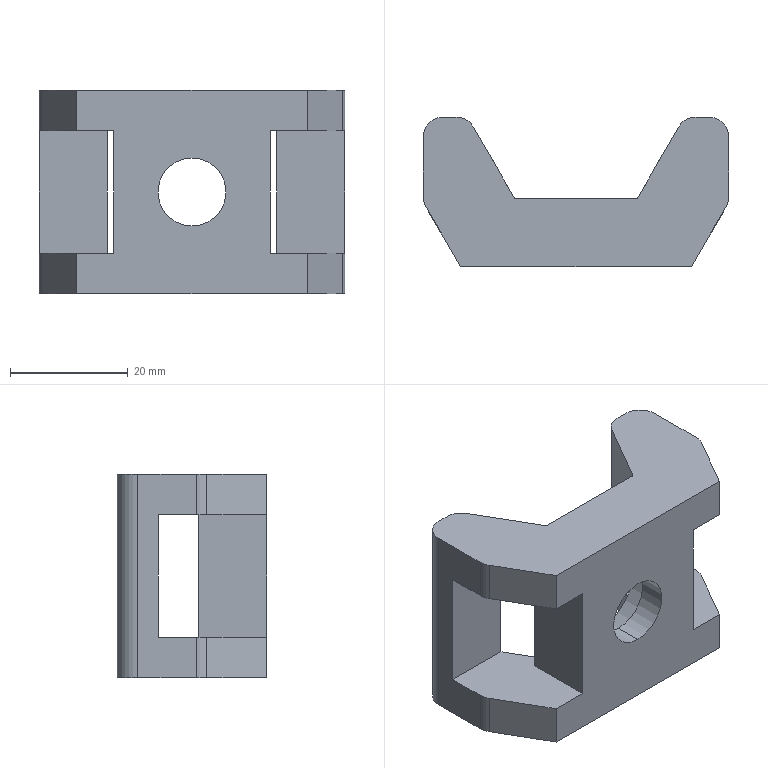Part | SolidWorks | features BaseBody 1 | 1 solid | 39 faces | box 51.923 x 25.385 x 34.615 mm | volume 17275 mm3 | plane 23 | cylinder 16 | commonest cylinder face diameters 6.923 x8 0.923 x4 11.538 x2 23.077 x2
STEP:
#1=CARTESIAN_POINT('',(57.247,363.731,113.462));
#2=VERTEX_POINT('',#1);
#3=CARTESIAN_POINT('',(57.247,363.731,101.923));
#4=VERTEX_POINT('',#3);
#5=CARTESIAN_POINT('',(57.247,363.731,107.692));
#6=DIRECTION('',(0.,-1.,0.));
#7=DIRECTION('',(0.,0.,1.));
#8=AXIS2_PLACEMENT_3D('',#5,#6,#7);
#9=CIRCLE('',#8,5.769);
#10=EDGE_CURVE('',#2,#4,#9,.T.);
#11=ORIENTED_EDGE('',*,*,#10,.T.);
#12=CARTESIAN_POINT('',(57.247,368.346,101.923));
#13=VERTEX_POINT('',#12);
#14=CARTESIAN_POINT('',(57.247,363.731,101.923));
#15=DIRECTION('',(0.,1.,0.));
#16=VECTOR('',#15,1000.);
#17=LINE('',#14,#16);
#18=EDGE_CURVE('',#4,#13,#17,.T.);
#19=ORIENTED_EDGE('',*,*,#18,.T.);
#20=CARTESIAN_POINT('',(57.247,368.346,113.462));
#21=VERTEX_POINT('',#20);
#22=CARTESIAN_POINT('',(57.247,368.346,107.692));
#23=DIRECTION('',(0.,-1.,0.));
#24=DIRECTION('',(0.,0.,1.));
#25=AXIS2_PLACEMENT_3D('',#22,#23,#24);
#26=CIRCLE('',#25,5.769);
#27=EDGE_CURVE('',#21,#13,#26,.T.);
#28=ORIENTED_EDGE('',*,*,#27,.F.);
#29=CARTESIAN_POINT('',(57.247,363.731,113.462));
#30=DIRECTION('',(0.,1.,0.));
#31=VECTOR('',#30,1000.);
#32=LINE('',#29,#31);
#33=EDGE_CURVE('',#2,#21,#32,.T.);
#34=ORIENTED_EDGE('',*,*,#33,.F.);
#35=EDGE_LOOP('',(#11,#19,#28,#34));
#36=FACE_OUTER_BOUND('',#35,.T.);
#37=CARTESIAN_POINT('',(57.247,363.731,107.692));
#38=DIRECTION('',(0.,1.,0.));
#39=DIRECTION('',(0.,0.,1.));
#40=AXIS2_PLACEMENT_3D('',#37,#38,#39);
#41=CYLINDRICAL_SURFACE('',#40,5.769);
#42=ADVANCED_FACE('',(#36),#41,.F.);
#43=CARTESIAN_POINT('',(57.247,368.346,96.154));
#44=VERTEX_POINT('',#43);
#45=CARTESIAN_POINT('',(57.247,368.346,119.231));
#46=VERTEX_POINT('',#45);
#47=CARTESIAN_POINT('',(57.247,368.346,107.692));
#48=DIRECTION('',(0.,1.,0.));
#49=DIRECTION('',(0.,0.,1.));
#50=AXIS2_PLACEMENT_3D('',#47,#48,#49);
#51=CIRCLE('',#50,11.538);
#52=EDGE_CURVE('',#44,#46,#51,.T.);
#53=ORIENTED_EDGE('',*,*,#52,.F.);
#54=CARTESIAN_POINT('',(57.247,375.269,96.154));
#55=VERTEX_POINT('',#54);
#56=CARTESIAN_POINT('',(57.247,363.731,96.154));
#57=DIRECTION('',(0.,1.,0.));
#58=VECTOR('',#57,1000.);
#59=LINE('',#56,#58);
#60=EDGE_CURVE('',#44,#55,#59,.T.);
#61=ORIENTED_EDGE('',*,*,#60,.T.);
#62=CARTESIAN_POINT('',(57.247,375.269,119.231));
#63=VERTEX_POINT('',#62);
#64=CARTESIAN_POINT('',(57.247,375.269,107.692));
#65=DIRECTION('',(0.,1.,0.));
#66=DIRECTION('',(0.,0.,1.));
#67=AXIS2_PLACEMENT_3D('',#64,#65,#66);
#68=CIRCLE('',#67,11.538);
#69=EDGE_CURVE('',#55,#63,#68,.T.);
#70=ORIENTED_EDGE('',*,*,#69,.T.);
#71=CARTESIAN_POINT('',(57.247,363.731,119.231));
#72=DIRECTION('',(0.,1.,0.));
#73=VECTOR('',#72,1000.);
#74=LINE('',#71,#73);
#75=EDGE_CURVE('',#46,#63,#74,.T.);
#76=ORIENTED_EDGE('',*,*,#75,.F.);
#77=EDGE_LOOP('',(#53,#61,#70,#76));
#78=FACE_OUTER_BOUND('',#77,.T.);
#79=CARTESIAN_POINT('',(57.247,363.731,107.692));
#80=DIRECTION('',(0.,1.,0.));
#81=DIRECTION('',(0.,0.,1.));
#82=AXIS2_PLACEMENT_3D('',#79,#80,#81);
#83=CYLINDRICAL_SURFACE('',#82,11.538);
#84=ADVANCED_FACE('',(#78),#83,.F.);
#85=ORIENTED_EDGE('',*,*,#10,.F.);
#86=CARTESIAN_POINT('',(57.247,363.731,107.692));
#87=DIRECTION('',(0.,-1.,0.));
#88=DIRECTION('',(0.,0.,1.));
#89=AXIS2_PLACEMENT_3D('',#86,#87,#88);
#90=CIRCLE('',#89,5.769);
#91=EDGE_CURVE('',#4,#2,#90,.T.);
#92=ORIENTED_EDGE('',*,*,#91,.F.);
#93=EDGE_LOOP('',(#85,#92));
#94=FACE_BOUND('',#93,.T.);
#95=CARTESIAN_POINT('',(76.862,363.731,118.077));
#96=VERTEX_POINT('',#95);
#97=CARTESIAN_POINT('',(70.516,363.731,118.077));
#98=VERTEX_POINT('',#97);
#99=CARTESIAN_POINT('',(37.631,363.731,118.077));
#100=DIRECTION('',(-1.,0.,0.));
#101=VECTOR('',#100,1000.);
#102=LINE('',#99,#101);
#103=EDGE_CURVE('',#96,#98,#102,.T.);
#104=ORIENTED_EDGE('',*,*,#103,.F.);
#105=CARTESIAN_POINT('',(76.862,363.731,125.));
#106=VERTEX_POINT('',#105);
#107=CARTESIAN_POINT('',(76.862,363.731,125.));
#108=DIRECTION('',(0.,0.,-1.));
#109=VECTOR('',#108,1000.);
#110=LINE('',#107,#109);
#111=EDGE_CURVE('',#106,#96,#110,.T.);
#112=ORIENTED_EDGE('',*,*,#111,.F.);
#113=CARTESIAN_POINT('',(37.631,363.731,125.));
#114=VERTEX_POINT('',#113);
#115=CARTESIAN_POINT('',(37.631,363.731,125.));
#116=DIRECTION('',(1.,0.,0.));
#117=VECTOR('',#116,1000.);
#118=LINE('',#115,#117);
#119=EDGE_CURVE('',#114,#106,#118,.T.);
#120=ORIENTED_EDGE('',*,*,#119,.F.);
#121=CARTESIAN_POINT('',(37.631,363.731,118.077));
#122=VERTEX_POINT('',#121);
#123=CARTESIAN_POINT('',(37.631,363.731,125.));
#124=DIRECTION('',(0.,0.,1.));
#125=VECTOR('',#124,1000.);
#126=LINE('',#123,#125);
#127=EDGE_CURVE('',#122,#114,#126,.T.);
#128=ORIENTED_EDGE('',*,*,#127,.F.);
#129=CARTESIAN_POINT('',(43.977,363.731,118.077));
#130=VERTEX_POINT('',#129);
#131=CARTESIAN_POINT('',(37.631,363.731,118.077));
#132=DIRECTION('',(-1.,0.,0.));
#133=VECTOR('',#132,1000.);
#134=LINE('',#131,#133);
#135=EDGE_CURVE('',#130,#122,#134,.T.);
#136=ORIENTED_EDGE('',*,*,#135,.F.);
#137=CARTESIAN_POINT('',(43.977,363.731,97.308));
#138=VERTEX_POINT('',#137);
#139=CARTESIAN_POINT('',(43.977,363.731,125.));
#140=DIRECTION('',(0.,0.,1.));
#141=VECTOR('',#140,1000.);
#142=LINE('',#139,#141);
#143=EDGE_CURVE('',#138,#130,#142,.T.);
#144=ORIENTED_EDGE('',*,*,#143,.F.);
#145=CARTESIAN_POINT('',(37.631,363.731,97.308));
#146=VERTEX_POINT('',#145);
#147=CARTESIAN_POINT('',(37.631,363.731,97.308));
#148=DIRECTION('',(1.,0.,0.));
#149=VECTOR('',#148,1000.);
#150=LINE('',#147,#149);
#151=EDGE_CURVE('',#146,#138,#150,.T.);
#152=ORIENTED_EDGE('',*,*,#151,.F.);
#153=CARTESIAN_POINT('',(37.631,363.731,90.385));
#154=VERTEX_POINT('',#153);
#155=CARTESIAN_POINT('',(37.631,363.731,125.));
#156=DIRECTION('',(0.,0.,1.));
#157=VECTOR('',#156,1000.);
#158=LINE('',#155,#157);
#159=EDGE_CURVE('',#154,#146,#158,.T.);
#160=ORIENTED_EDGE('',*,*,#159,.F.);
#161=CARTESIAN_POINT('',(76.862,363.731,90.385));
#162=VERTEX_POINT('',#161);
#163=CARTESIAN_POINT('',(37.631,363.731,90.385));
#164=DIRECTION('',(-1.,0.,0.));
#165=VECTOR('',#164,1000.);
#166=LINE('',#163,#165);
#167=EDGE_CURVE('',#162,#154,#166,.T.);
#168=ORIENTED_EDGE('',*,*,#167,.F.);
#169=CARTESIAN_POINT('',(76.862,363.731,97.308));
#170=VERTEX_POINT('',#169);
#171=CARTESIAN_POINT('',(76.862,363.731,125.));
#172=DIRECTION('',(0.,0.,-1.));
#173=VECTOR('',#172,1000.);
#174=LINE('',#171,#173);
#175=EDGE_CURVE('',#170,#162,#174,.T.);
#176=ORIENTED_EDGE('',*,*,#175,.F.);
#177=CARTESIAN_POINT('',(70.516,363.731,97.308));
#178=VERTEX_POINT('',#177);
#179=CARTESIAN_POINT('',(37.631,363.731,97.308));
#180=DIRECTION('',(1.,0.,0.));
#181=VECTOR('',#180,1000.);
#182=LINE('',#179,#181);
#183=EDGE_CURVE('',#178,#170,#182,.T.);
#184=ORIENTED_EDGE('',*,*,#183,.F.);
#185=CARTESIAN_POINT('',(70.516,363.731,125.));
#186=DIRECTION('',(0.,0.,-1.));
#187=VECTOR('',#186,1000.);
#188=LINE('',#185,#187);
#189=EDGE_CURVE('',#98,#178,#188,.T.);
#190=ORIENTED_EDGE('',*,*,#189,.F.);
#191=EDGE_LOOP('',(#104,#112,#120,#128,#136,#144,#152,#160,#168,#176,#184,#190));
#192=FACE_OUTER_BOUND('',#191,.T.);
#193=CARTESIAN_POINT('',(37.631,363.731,125.));
#194=DIRECTION('',(0.,1.,0.));
#195=DIRECTION('',(0.,0.,1.));
#196=AXIS2_PLACEMENT_3D('',#193,#194,#195);
#197=PLANE('',#196);
#198=ADVANCED_FACE('',(#94,#192),#197,.F.);
#199=ORIENTED_EDGE('',*,*,#18,.F.);
#200=ORIENTED_EDGE('',*,*,#91,.T.);
#201=ORIENTED_EDGE('',*,*,#33,.T.);
#202=CARTESIAN_POINT('',(57.247,368.346,107.692));
#203=DIRECTION('',(0.,-1.,0.));
#204=DIRECTION('',(0.,0.,1.));
#205=AXIS2_PLACEMENT_3D('',#202,#203,#204);
#206=CIRCLE('',#205,5.769);
#207=EDGE_CURVE('',#13,#21,#206,.T.);
#208=ORIENTED_EDGE('',*,*,#207,.F.);
#209=EDGE_LOOP('',(#199,#200,#201,#208));
#210=FACE_OUTER_BOUND('',#209,.T.);
#211=CARTESIAN_POINT('',(57.247,363.731,107.692));
#212=DIRECTION('',(0.,1.,0.));
#213=DIRECTION('',(0.,0.,1.));
#214=AXIS2_PLACEMENT_3D('',#211,#212,#213);
#215=CYLINDRICAL_SURFACE('',#214,5.769);
#216=ADVANCED_FACE('',(#210),#215,.F.);
#217=ORIENTED_EDGE('',*,*,#189,.T.);
#218=CARTESIAN_POINT('',(70.516,375.269,97.308));
#219=VERTEX_POINT('',#218);
#220=CARTESIAN_POINT('',(70.516,375.269,97.308));
#221=DIRECTION('',(0.,-1.,0.));
#222=VECTOR('',#221,1000.);
#223=LINE('',#220,#222);
#224=EDGE_CURVE('',#219,#178,#223,.T.);
#225=ORIENTED_EDGE('',*,*,#224,.F.);
#226=CARTESIAN_POINT('',(70.516,375.269,118.077));
#227=VERTEX_POINT('',#226);
#228=CARTESIAN_POINT('',(70.516,375.269,118.077));
#229=DIRECTION('',(0.,0.,-1.));
#230=VECTOR('',#229,1000.);
#231=LINE('',#228,#230);
#232=EDGE_CURVE('',#227,#219,#231,.T.);
#233=ORIENTED_EDGE('',*,*,#232,.F.);
#234=CARTESIAN_POINT('',(70.516,375.269,118.077));
#235=DIRECTION('',(0.,1.,0.));
#236=VECTOR('',#235,1000.);
#237=LINE('',#234,#236);
#238=EDGE_CURVE('',#98,#227,#237,.T.);
#239=ORIENTED_EDGE('',*,*,#238,.F.);
#240=EDGE_LOOP('',(#217,#225,#233,#239));
#241=FACE_OUTER_BOUND('',#240,.T.);
#242=CARTESIAN_POINT('',(70.516,375.269,118.077));
#243=DIRECTION('',(-1.,0.,0.));
#244=DIRECTION('',(0.,0.,1.));
#245=AXIS2_PLACEMENT_3D('',#242,#243,#244);
#246=PLANE('',#245);
#247=ADVANCED_FACE('',(#241),#246,.F.);
#248=CARTESIAN_POINT('',(67.775,375.5,118.077));
#249=VERTEX_POINT('',#248);
#250=CARTESIAN_POINT('',(71.639,382.192,118.077));
#251=VERTEX_POINT('',#250);
#252=CARTESIAN_POINT('',(67.775,375.5,118.077));
#253=DIRECTION('',(0.5,0.866,0.));
#254=VECTOR('',#253,1000.);
#255=LINE('',#252,#254);
#256=EDGE_CURVE('',#249,#251,#255,.T.);
#257=ORIENTED_EDGE('',*,*,#256,.T.);
#258=CARTESIAN_POINT('',(83.208,382.192,118.077));
#259=VERTEX_POINT('',#258);
#260=CARTESIAN_POINT('',(91.862,382.192,118.077));
#261=DIRECTION('',(1.,0.,0.));
#262=VECTOR('',#261,1000.);
#263=LINE('',#260,#262);
#264=EDGE_CURVE('',#251,#259,#263,.T.);
#265=ORIENTED_EDGE('',*,*,#264,.T.);
#266=CARTESIAN_POINT('',(83.208,375.65,118.077));
#267=VERTEX_POINT('',#266);
#268=CARTESIAN_POINT('',(83.208,382.192,118.077));
#269=DIRECTION('',(0.,-1.,0.));
#270=VECTOR('',#269,1000.);
#271=LINE('',#268,#270);
#272=EDGE_CURVE('',#259,#267,#271,.T.);
#273=ORIENTED_EDGE('',*,*,#272,.T.);
#274=CARTESIAN_POINT('',(82.744,373.919,118.077));
#275=VERTEX_POINT('',#274);
#276=CARTESIAN_POINT('',(79.747,375.65,118.077));
#277=DIRECTION('',(0.,0.,-1.));
#278=DIRECTION('',(1.,0.,0.));
#279=AXIS2_PLACEMENT_3D('',#276,#277,#278);
#280=CIRCLE('',#279,3.462);
#281=EDGE_CURVE('',#267,#275,#280,.T.);
#282=ORIENTED_EDGE('',*,*,#281,.T.);
#283=CARTESIAN_POINT('',(82.744,373.919,118.077));
#284=DIRECTION('',(-0.5,-0.866,0.));
#285=VECTOR('',#284,1000.);
#286=LINE('',#283,#285);
#287=EDGE_CURVE('',#275,#96,#286,.T.);
#288=ORIENTED_EDGE('',*,*,#287,.T.);
#289=ORIENTED_EDGE('',*,*,#103,.T.);
#290=ORIENTED_EDGE('',*,*,#238,.T.);
#291=CARTESIAN_POINT('',(67.376,375.269,118.077));
#292=VERTEX_POINT('',#291);
#293=CARTESIAN_POINT('',(91.862,375.269,118.077));
#294=DIRECTION('',(-1.,0.,0.));
#295=VECTOR('',#294,1000.);
#296=LINE('',#293,#295);
#297=EDGE_CURVE('',#227,#292,#296,.T.);
#298=ORIENTED_EDGE('',*,*,#297,.T.);
#299=CARTESIAN_POINT('',(67.376,375.731,118.077));
#300=DIRECTION('',(0.,0.,1.));
#301=DIRECTION('',(1.,0.,0.));
#302=AXIS2_PLACEMENT_3D('',#299,#300,#301);
#303=CIRCLE('',#302,0.4615);
#304=EDGE_CURVE('',#292,#249,#303,.T.);
#305=ORIENTED_EDGE('',*,*,#304,.T.);
#306=EDGE_LOOP('',(#257,#265,#273,#282,#288,#289,#290,#298,#305));
#307=FACE_OUTER_BOUND('',#306,.T.);
#308=CARTESIAN_POINT('',(91.862,382.192,118.077));
#309=DIRECTION('',(0.,0.,-1.));
#310=DIRECTION('',(-1.,0.,0.));
#311=AXIS2_PLACEMENT_3D('',#308,#309,#310);
#312=PLANE('',#311);
#313=ADVANCED_FACE('',(#307),#312,.T.);
#314=CARTESIAN_POINT('',(82.744,373.919,125.));
#315=VERTEX_POINT('',#314);
#316=CARTESIAN_POINT('',(76.862,363.731,125.));
#317=DIRECTION('',(0.5,0.866,0.));
#318=VECTOR('',#317,1000.);
#319=LINE('',#316,#318);
#320=EDGE_CURVE('',#106,#315,#319,.T.);
#321=ORIENTED_EDGE('',*,*,#320,.F.);
#322=ORIENTED_EDGE('',*,*,#111,.T.);
#323=ORIENTED_EDGE('',*,*,#287,.F.);
#324=CARTESIAN_POINT('',(82.744,373.919,125.));
#325=DIRECTION('',(0.,0.,-1.));
#326=VECTOR('',#325,1000.);
#327=LINE('',#324,#326);
#328=EDGE_CURVE('',#315,#275,#327,.T.);
#329=ORIENTED_EDGE('',*,*,#328,.F.);
#330=EDGE_LOOP('',(#321,#322,#323,#329));
#331=FACE_OUTER_BOUND('',#330,.T.);
#332=CARTESIAN_POINT('',(76.862,363.731,125.));
#333=DIRECTION('',(-0.866,0.5,0.));
#334=DIRECTION('',(-0.5,-0.866,0.));
#335=AXIS2_PLACEMENT_3D('',#332,#333,#334);
#336=PLANE('',#335);
#337=ADVANCED_FACE('',(#331),#336,.F.);
#338=CARTESIAN_POINT('',(39.856,387.385,125.));
#339=VERTEX_POINT('',#338);
#340=CARTESIAN_POINT('',(36.858,389.115,125.));
#341=VERTEX_POINT('',#340);
#342=CARTESIAN_POINT('',(36.858,385.654,125.));
#343=DIRECTION('',(0.,0.,1.));
#344=DIRECTION('',(1.,0.,0.));
#345=AXIS2_PLACEMENT_3D('',#342,#343,#344);
#346=CIRCLE('',#345,3.462);
#347=EDGE_CURVE('',#339,#341,#346,.T.);
#348=ORIENTED_EDGE('',*,*,#347,.T.);
#349=CARTESIAN_POINT('',(34.747,389.115,125.));
#350=VERTEX_POINT('',#349);
#351=CARTESIAN_POINT('',(34.747,389.115,125.));
#352=DIRECTION('',(-1.,0.,0.));
#353=VECTOR('',#352,1000.);
#354=LINE('',#351,#353);
#355=EDGE_CURVE('',#341,#350,#354,.T.);
#356=ORIENTED_EDGE('',*,*,#355,.T.);
#357=CARTESIAN_POINT('',(31.285,385.654,125.));
#358=VERTEX_POINT('',#357);
#359=CARTESIAN_POINT('',(34.747,385.654,125.));
#360=DIRECTION('',(0.,0.,1.));
#361=DIRECTION('',(1.,0.,0.));
#362=AXIS2_PLACEMENT_3D('',#359,#360,#361);
#363=CIRCLE('',#362,3.462);
#364=EDGE_CURVE('',#350,#358,#363,.T.);
#365=ORIENTED_EDGE('',*,*,#364,.T.);
#366=CARTESIAN_POINT('',(31.285,375.65,125.));
#367=VERTEX_POINT('',#366);
#368=CARTESIAN_POINT('',(31.285,375.65,125.));
#369=DIRECTION('',(0.,-1.,0.));
#370=VECTOR('',#369,1000.);
#371=LINE('',#368,#370);
#372=EDGE_CURVE('',#358,#367,#371,.T.);
#373=ORIENTED_EDGE('',*,*,#372,.T.);
#374=CARTESIAN_POINT('',(31.749,373.919,125.));
#375=VERTEX_POINT('',#374);
#376=CARTESIAN_POINT('',(34.747,375.65,125.));
#377=DIRECTION('',(0.,0.,1.));
#378=DIRECTION('',(1.,0.,0.));
#379=AXIS2_PLACEMENT_3D('',#376,#377,#378);
#380=CIRCLE('',#379,3.462);
#381=EDGE_CURVE('',#367,#375,#380,.T.);
#382=ORIENTED_EDGE('',*,*,#381,.T.);
#383=CARTESIAN_POINT('',(31.749,373.919,125.));
#384=DIRECTION('',(0.5,-0.866,0.));
#385=VECTOR('',#384,1000.);
#386=LINE('',#383,#385);
#387=EDGE_CURVE('',#375,#114,#386,.T.);
#388=ORIENTED_EDGE('',*,*,#387,.T.);
#389=ORIENTED_EDGE('',*,*,#119,.T.);
#390=ORIENTED_EDGE('',*,*,#320,.T.);
#391=CARTESIAN_POINT('',(83.208,375.65,125.));
#392=VERTEX_POINT('',#391);
#393=CARTESIAN_POINT('',(79.747,375.65,125.));
#394=DIRECTION('',(0.,0.,1.));
#395=DIRECTION('',(1.,0.,0.));
#396=AXIS2_PLACEMENT_3D('',#393,#394,#395);
#397=CIRCLE('',#396,3.462);
#398=EDGE_CURVE('',#315,#392,#397,.T.);
#399=ORIENTED_EDGE('',*,*,#398,.T.);
#400=CARTESIAN_POINT('',(83.208,385.654,125.));
#401=VERTEX_POINT('',#400);
#402=CARTESIAN_POINT('',(83.208,375.65,125.));
#403=DIRECTION('',(0.,1.,0.));
#404=VECTOR('',#403,1000.);
#405=LINE('',#402,#404);
#406=EDGE_CURVE('',#392,#401,#405,.T.);
#407=ORIENTED_EDGE('',*,*,#406,.T.);
#408=CARTESIAN_POINT('',(79.747,389.115,125.));
#409=VERTEX_POINT('',#408);
#410=CARTESIAN_POINT('',(79.747,385.654,125.));
#411=DIRECTION('',(0.,0.,1.));
#412=DIRECTION('',(1.,0.,0.));
#413=AXIS2_PLACEMENT_3D('',#410,#411,#412);
#414=CIRCLE('',#413,3.462);
#415=EDGE_CURVE('',#401,#409,#414,.T.);
#416=ORIENTED_EDGE('',*,*,#415,.T.);
#417=CARTESIAN_POINT('',(77.635,389.115,125.));
#418=VERTEX_POINT('',#417);
#419=CARTESIAN_POINT('',(34.747,389.115,125.));
#420=DIRECTION('',(-1.,0.,0.));
#421=VECTOR('',#420,1000.);
#422=LINE('',#419,#421);
#423=EDGE_CURVE('',#409,#418,#422,.T.);
#424=ORIENTED_EDGE('',*,*,#423,.T.);
#425=CARTESIAN_POINT('',(74.637,387.385,125.));
#426=VERTEX_POINT('',#425);
#427=CARTESIAN_POINT('',(77.635,385.654,125.));
#428=DIRECTION('',(0.,0.,1.));
#429=DIRECTION('',(1.,0.,0.));
#430=AXIS2_PLACEMENT_3D('',#427,#428,#429);
#431=CIRCLE('',#430,3.462);
#432=EDGE_CURVE('',#418,#426,#431,.T.);
#433=ORIENTED_EDGE('',*,*,#432,.T.);
#434=CARTESIAN_POINT('',(67.775,375.5,125.));
#435=VERTEX_POINT('',#434);
#436=CARTESIAN_POINT('',(74.637,387.385,125.));
#437=DIRECTION('',(-0.5,-0.866,0.));
#438=VECTOR('',#437,1000.);
#439=LINE('',#436,#438);
#440=EDGE_CURVE('',#426,#435,#439,.T.);
#441=ORIENTED_EDGE('',*,*,#440,.T.);
#442=CARTESIAN_POINT('',(67.376,375.269,125.));
#443=VERTEX_POINT('',#442);
#444=CARTESIAN_POINT('',(67.376,375.731,125.));
#445=DIRECTION('',(0.,0.,-1.));
#446=DIRECTION('',(1.,0.,0.));
#447=AXIS2_PLACEMENT_3D('',#444,#445,#446);
#448=CIRCLE('',#447,0.4615);
#449=EDGE_CURVE('',#435,#443,#448,.T.);
#450=ORIENTED_EDGE('',*,*,#449,.T.);
#451=CARTESIAN_POINT('',(47.117,375.269,125.));
#452=VERTEX_POINT('',#451);
#453=CARTESIAN_POINT('',(34.747,375.269,125.));
#454=DIRECTION('',(-1.,0.,0.));
#455=VECTOR('',#454,1000.);
#456=LINE('',#453,#455);
#457=EDGE_CURVE('',#443,#452,#456,.T.);
#458=ORIENTED_EDGE('',*,*,#457,.T.);
#459=CARTESIAN_POINT('',(46.718,375.5,125.));
#460=VERTEX_POINT('',#459);
#461=CARTESIAN_POINT('',(47.117,375.731,125.));
#462=DIRECTION('',(0.,0.,-1.));
#463=DIRECTION('',(1.,0.,0.));
#464=AXIS2_PLACEMENT_3D('',#461,#462,#463);
#465=CIRCLE('',#464,0.4615);
#466=EDGE_CURVE('',#452,#460,#465,.T.);
#467=ORIENTED_EDGE('',*,*,#466,.T.);
#468=CARTESIAN_POINT('',(46.718,375.5,125.));
#469=DIRECTION('',(-0.5,0.866,0.));
#470=VECTOR('',#469,1000.);
#471=LINE('',#468,#470);
#472=EDGE_CURVE('',#460,#339,#471,.T.);
#473=ORIENTED_EDGE('',*,*,#472,.T.);
#474=EDGE_LOOP('',(#348,#356,#365,#373,#382,#388,#389,#390,#399,#407,#416,#424,#433,#441,#450,#458,#467,#473));
#475=FACE_OUTER_BOUND('',#474,.T.);
#476=CARTESIAN_POINT('',(34.747,375.65,125.));
#477=DIRECTION('',(0.,0.,1.));
#478=DIRECTION('',(1.,0.,0.));
#479=AXIS2_PLACEMENT_3D('',#476,#477,#478);
#480=PLANE('',#479);
#481=ADVANCED_FACE('',(#475),#480,.T.);
#482=ORIENTED_EDGE('',*,*,#387,.F.);
#483=CARTESIAN_POINT('',(31.749,373.919,118.077));
#484=VERTEX_POINT('',#483);
#485=CARTESIAN_POINT('',(31.749,373.919,125.));
#486=DIRECTION('',(0.,0.,1.));
#487=VECTOR('',#486,1000.);
#488=LINE('',#485,#487);
#489=EDGE_CURVE('',#484,#375,#488,.T.);
#490=ORIENTED_EDGE('',*,*,#489,.F.);
#491=CARTESIAN_POINT('',(31.749,373.919,118.077));
#492=DIRECTION('',(-0.5,0.866,0.));
#493=VECTOR('',#492,1000.);
#494=LINE('',#491,#493);
#495=EDGE_CURVE('',#122,#484,#494,.T.);
#496=ORIENTED_EDGE('',*,*,#495,.F.);
#497=ORIENTED_EDGE('',*,*,#127,.T.);
#498=EDGE_LOOP('',(#482,#490,#496,#497));
#499=FACE_OUTER_BOUND('',#498,.T.);
#500=CARTESIAN_POINT('',(31.749,373.919,125.));
#501=DIRECTION('',(0.866,0.5,0.));
#502=DIRECTION('',(-0.5,0.866,0.));
#503=AXIS2_PLACEMENT_3D('',#500,#501,#502);
#504=PLANE('',#503);
#505=ADVANCED_FACE('',(#499),#504,.F.);
#506=ORIENTED_EDGE('',*,*,#135,.T.);
#507=ORIENTED_EDGE('',*,*,#495,.T.);
#508=CARTESIAN_POINT('',(31.285,375.65,118.077));
#509=VERTEX_POINT('',#508);
#510=CARTESIAN_POINT('',(34.747,375.65,118.077));
#511=DIRECTION('',(0.,0.,-1.));
#512=DIRECTION('',(1.,0.,0.));
#513=AXIS2_PLACEMENT_3D('',#510,#511,#512);
#514=CIRCLE('',#513,3.462);
#515=EDGE_CURVE('',#484,#509,#514,.T.);
#516=ORIENTED_EDGE('',*,*,#515,.T.);
#517=CARTESIAN_POINT('',(31.285,382.192,118.077));
#518=VERTEX_POINT('',#517);
#519=CARTESIAN_POINT('',(31.285,382.192,118.077));
#520=DIRECTION('',(0.,1.,0.));
#521=VECTOR('',#520,1000.);
#522=LINE('',#519,#521);
#523=EDGE_CURVE('',#509,#518,#522,.T.);
#524=ORIENTED_EDGE('',*,*,#523,.T.);
#525=CARTESIAN_POINT('',(42.854,382.192,118.077));
#526=VERTEX_POINT('',#525);
#527=CARTESIAN_POINT('',(91.862,382.192,118.077));
#528=DIRECTION('',(1.,0.,0.));
#529=VECTOR('',#528,1000.);
#530=LINE('',#527,#529);
#531=EDGE_CURVE('',#518,#526,#530,.T.);
#532=ORIENTED_EDGE('',*,*,#531,.T.);
#533=CARTESIAN_POINT('',(46.718,375.5,118.077));
#534=VERTEX_POINT('',#533);
#535=CARTESIAN_POINT('',(42.854,382.192,118.077));
#536=DIRECTION('',(0.5,-0.866,0.));
#537=VECTOR('',#536,1000.);
#538=LINE('',#535,#537);
#539=EDGE_CURVE('',#526,#534,#538,.T.);
#540=ORIENTED_EDGE('',*,*,#539,.T.);
#541=CARTESIAN_POINT('',(47.117,375.269,118.077));
#542=VERTEX_POINT('',#541);
#543=CARTESIAN_POINT('',(47.117,375.731,118.077));
#544=DIRECTION('',(0.,0.,1.));
#545=DIRECTION('',(1.,0.,0.));
#546=AXIS2_PLACEMENT_3D('',#543,#544,#545);
#547=CIRCLE('',#546,0.4615);
#548=EDGE_CURVE('',#534,#542,#547,.T.);
#549=ORIENTED_EDGE('',*,*,#548,.T.);
#550=CARTESIAN_POINT('',(43.977,375.269,118.077));
#551=VERTEX_POINT('',#550);
#552=CARTESIAN_POINT('',(91.862,375.269,118.077));
#553=DIRECTION('',(-1.,0.,0.));
#554=VECTOR('',#553,1000.);
#555=LINE('',#552,#554);
#556=EDGE_CURVE('',#542,#551,#555,.T.);
#557=ORIENTED_EDGE('',*,*,#556,.T.);
#558=CARTESIAN_POINT('',(43.977,382.192,118.077));
#559=DIRECTION('',(0.,-1.,0.));
#560=VECTOR('',#559,1000.);
#561=LINE('',#558,#560);
#562=EDGE_CURVE('',#551,#130,#561,.T.);
#563=ORIENTED_EDGE('',*,*,#562,.T.);
#564=EDGE_LOOP('',(#506,#507,#516,#524,#532,#540,#549,#557,#563));
#565=FACE_OUTER_BOUND('',#564,.T.);
#566=CARTESIAN_POINT('',(91.862,382.192,118.077));
#567=DIRECTION('',(0.,0.,-1.));
#568=DIRECTION('',(-1.,0.,0.));
#569=AXIS2_PLACEMENT_3D('',#566,#567,#568);
#570=PLANE('',#569);
#571=ADVANCED_FACE('',(#565),#570,.T.);
#572=ORIENTED_EDGE('',*,*,#143,.T.);
#573=ORIENTED_EDGE('',*,*,#562,.F.);
#574=CARTESIAN_POINT('',(43.977,375.269,97.308));
#575=VERTEX_POINT('',#574);
#576=CARTESIAN_POINT('',(43.977,375.269,97.308));
#577=DIRECTION('',(0.,0.,1.));
#578=VECTOR('',#577,1000.);
#579=LINE('',#576,#578);
#580=EDGE_CURVE('',#575,#551,#579,.T.);
#581=ORIENTED_EDGE('',*,*,#580,.F.);
#582=CARTESIAN_POINT('',(43.977,375.269,97.308));
#583=DIRECTION('',(0.,1.,0.));
#584=VECTOR('',#583,1000.);
#585=LINE('',#582,#584);
#586=EDGE_CURVE('',#138,#575,#585,.T.);
#587=ORIENTED_EDGE('',*,*,#586,.F.);
#588=EDGE_LOOP('',(#572,#573,#581,#587));
#589=FACE_OUTER_BOUND('',#588,.T.);
#590=CARTESIAN_POINT('',(43.977,375.269,97.308));
#591=DIRECTION('',(1.,0.,0.));
#592=DIRECTION('',(0.,0.,-1.));
#593=AXIS2_PLACEMENT_3D('',#590,#591,#592);
#594=PLANE('',#593);
#595=ADVANCED_FACE('',(#589),#594,.F.);
#596=CARTESIAN_POINT('',(47.117,375.269,97.308));
#597=VERTEX_POINT('',#596);
#598=CARTESIAN_POINT('',(46.718,375.5,97.308));
#599=VERTEX_POINT('',#598);
#600=CARTESIAN_POINT('',(47.117,375.731,97.308));
#601=DIRECTION('',(0.,0.,-1.));
#602=DIRECTION('',(1.,0.,0.));
#603=AXIS2_PLACEMENT_3D('',#600,#601,#602);
#604=CIRCLE('',#603,0.4615);
#605=EDGE_CURVE('',#597,#599,#604,.T.);
#606=ORIENTED_EDGE('',*,*,#605,.T.);
#607=CARTESIAN_POINT('',(42.854,382.192,97.308));
#608=VERTEX_POINT('',#607);
#609=CARTESIAN_POINT('',(46.718,375.5,97.308));
#610=DIRECTION('',(-0.5,0.866,0.));
#611=VECTOR('',#610,1000.);
#612=LINE('',#609,#611);
#613=EDGE_CURVE('',#599,#608,#612,.T.);
#614=ORIENTED_EDGE('',*,*,#613,.T.);
#615=CARTESIAN_POINT('',(31.285,382.192,97.308));
#616=VERTEX_POINT('',#615);
#617=CARTESIAN_POINT('',(91.862,382.192,97.308));
#618=DIRECTION('',(-1.,0.,0.));
#619=VECTOR('',#618,1000.);
#620=LINE('',#617,#619);
#621=EDGE_CURVE('',#608,#616,#620,.T.);
#622=ORIENTED_EDGE('',*,*,#621,.T.);
#623=CARTESIAN_POINT('',(31.285,375.65,97.308));
#624=VERTEX_POINT('',#623);
#625=CARTESIAN_POINT('',(31.285,375.269,97.308));
#626=DIRECTION('',(0.,-1.,0.));
#627=VECTOR('',#626,1000.);
#628=LINE('',#625,#627);
#629=EDGE_CURVE('',#616,#624,#628,.T.);
#630=ORIENTED_EDGE('',*,*,#629,.T.);
#631=CARTESIAN_POINT('',(31.749,373.919,97.308));
#632=VERTEX_POINT('',#631);
#633=CARTESIAN_POINT('',(34.747,375.65,97.308));
#634=DIRECTION('',(0.,0.,1.));
#635=DIRECTION('',(1.,0.,0.));
#636=AXIS2_PLACEMENT_3D('',#633,#634,#635);
#637=CIRCLE('',#636,3.462);
#638=EDGE_CURVE('',#624,#632,#637,.T.);
#639=ORIENTED_EDGE('',*,*,#638,.T.);
#640=CARTESIAN_POINT('',(31.749,373.919,97.308));
#641=DIRECTION('',(0.5,-0.866,0.));
#642=VECTOR('',#641,1000.);
#643=LINE('',#640,#642);
#644=EDGE_CURVE('',#632,#146,#643,.T.);
#645=ORIENTED_EDGE('',*,*,#644,.T.);
#646=ORIENTED_EDGE('',*,*,#151,.T.);
#647=ORIENTED_EDGE('',*,*,#586,.T.);
#648=CARTESIAN_POINT('',(91.862,375.269,97.308));
#649=DIRECTION('',(1.,0.,0.));
#650=VECTOR('',#649,1000.);
#651=LINE('',#648,#650);
#652=EDGE_CURVE('',#575,#597,#651,.T.);
#653=ORIENTED_EDGE('',*,*,#652,.T.);
#654=EDGE_LOOP('',(#606,#614,#622,#630,#639,#645,#646,#647,#653));
#655=FACE_OUTER_BOUND('',#654,.T.);
#656=CARTESIAN_POINT('',(91.862,375.269,97.308));
#657=DIRECTION('',(0.,0.,1.));
#658=DIRECTION('',(1.,0.,0.));
#659=AXIS2_PLACEMENT_3D('',#656,#657,#658);
#660=PLANE('',#659);
#661=ADVANCED_FACE('',(#655),#660,.T.);
#662=CARTESIAN_POINT('',(31.749,373.919,90.385));
#663=VERTEX_POINT('',#662);
#664=CARTESIAN_POINT('',(31.749,373.919,90.385));
#665=DIRECTION('',(-0.5,0.866,0.));
#666=VECTOR('',#665,1000.);
#667=LINE('',#664,#666);
#668=EDGE_CURVE('',#154,#663,#667,.T.);
#669=ORIENTED_EDGE('',*,*,#668,.F.);
#670=ORIENTED_EDGE('',*,*,#159,.T.);
#671=ORIENTED_EDGE('',*,*,#644,.F.);
#672=CARTESIAN_POINT('',(31.749,373.919,125.));
#673=DIRECTION('',(0.,0.,1.));
#674=VECTOR('',#673,1000.);
#675=LINE('',#672,#674);
#676=EDGE_CURVE('',#663,#632,#675,.T.);
#677=ORIENTED_EDGE('',*,*,#676,.F.);
#678=EDGE_LOOP('',(#669,#670,#671,#677));
#679=FACE_OUTER_BOUND('',#678,.T.);
#680=CARTESIAN_POINT('',(31.749,373.919,125.));
#681=DIRECTION('',(0.866,0.5,0.));
#682=DIRECTION('',(-0.5,0.866,0.));
#683=AXIS2_PLACEMENT_3D('',#680,#681,#682);
#684=PLANE('',#683);
#685=ADVANCED_FACE('',(#679),#684,.F.);
#686=CARTESIAN_POINT('',(39.856,387.385,90.385));
#687=VERTEX_POINT('',#686);
#688=CARTESIAN_POINT('',(36.858,389.115,90.385));
#689=VERTEX_POINT('',#688);
#690=CARTESIAN_POINT('',(36.858,385.654,90.385));
#691=DIRECTION('',(0.,0.,1.));
#692=DIRECTION('',(1.,0.,0.));
#693=AXIS2_PLACEMENT_3D('',#690,#691,#692);
#694=CIRCLE('',#693,3.462);
#695=EDGE_CURVE('',#687,#689,#694,.T.);
#696=ORIENTED_EDGE('',*,*,#695,.F.);
#697=CARTESIAN_POINT('',(46.718,375.5,90.385));
#698=VERTEX_POINT('',#697);
#699=CARTESIAN_POINT('',(46.718,375.5,90.385));
#700=DIRECTION('',(-0.5,0.866,0.));
#701=VECTOR('',#700,1000.);
#702=LINE('',#699,#701);
#703=EDGE_CURVE('',#698,#687,#702,.T.);
#704=ORIENTED_EDGE('',*,*,#703,.F.);
#705=CARTESIAN_POINT('',(47.117,375.269,90.385));
#706=VERTEX_POINT('',#705);
#707=CARTESIAN_POINT('',(47.117,375.731,90.385));
#708=DIRECTION('',(0.,0.,-1.));
#709=DIRECTION('',(1.,0.,0.));
#710=AXIS2_PLACEMENT_3D('',#707,#708,#709);
#711=CIRCLE('',#710,0.4615);
#712=EDGE_CURVE('',#706,#698,#711,.T.);
#713=ORIENTED_EDGE('',*,*,#712,.F.);
#714=CARTESIAN_POINT('',(67.376,375.269,90.385));
#715=VERTEX_POINT('',#714);
#716=CARTESIAN_POINT('',(34.747,375.269,90.385));
#717=DIRECTION('',(-1.,0.,0.));
#718=VECTOR('',#717,1000.);
#719=LINE('',#716,#718);
#720=EDGE_CURVE('',#715,#706,#719,.T.);
#721=ORIENTED_EDGE('',*,*,#720,.F.);
#722=CARTESIAN_POINT('',(67.775,375.5,90.385));
#723=VERTEX_POINT('',#722);
#724=CARTESIAN_POINT('',(67.376,375.731,90.385));
#725=DIRECTION('',(0.,0.,-1.));
#726=DIRECTION('',(1.,0.,0.));
#727=AXIS2_PLACEMENT_3D('',#724,#725,#726);
#728=CIRCLE('',#727,0.4615);
#729=EDGE_CURVE('',#723,#715,#728,.T.);
#730=ORIENTED_EDGE('',*,*,#729,.F.);
#731=CARTESIAN_POINT('',(74.637,387.385,90.385));
#732=VERTEX_POINT('',#731);
#733=CARTESIAN_POINT('',(74.637,387.385,90.385));
#734=DIRECTION('',(-0.5,-0.866,0.));
#735=VECTOR('',#734,1000.);
#736=LINE('',#733,#735);
#737=EDGE_CURVE('',#732,#723,#736,.T.);
#738=ORIENTED_EDGE('',*,*,#737,.F.);
#739=CARTESIAN_POINT('',(77.635,389.115,90.385));
#740=VERTEX_POINT('',#739);
#741=CARTESIAN_POINT('',(77.635,385.654,90.385));
#742=DIRECTION('',(0.,0.,1.));
#743=DIRECTION('',(1.,0.,0.));
#744=AXIS2_PLACEMENT_3D('',#741,#742,#743);
#745=CIRCLE('',#744,3.462);
#746=EDGE_CURVE('',#740,#732,#745,.T.);
#747=ORIENTED_EDGE('',*,*,#746,.F.);
#748=CARTESIAN_POINT('',(79.747,389.115,90.385));
#749=VERTEX_POINT('',#748);
#750=CARTESIAN_POINT('',(34.747,389.115,90.385));
#751=DIRECTION('',(-1.,0.,0.));
#752=VECTOR('',#751,1000.);
#753=LINE('',#750,#752);
#754=EDGE_CURVE('',#749,#740,#753,.T.);
#755=ORIENTED_EDGE('',*,*,#754,.F.);
#756=CARTESIAN_POINT('',(83.208,385.654,90.385));
#757=VERTEX_POINT('',#756);
#758=CARTESIAN_POINT('',(79.747,385.654,90.385));
#759=DIRECTION('',(0.,0.,1.));
#760=DIRECTION('',(1.,0.,0.));
#761=AXIS2_PLACEMENT_3D('',#758,#759,#760);
#762=CIRCLE('',#761,3.462);
#763=EDGE_CURVE('',#757,#749,#762,.T.);
#764=ORIENTED_EDGE('',*,*,#763,.F.);
#765=CARTESIAN_POINT('',(83.208,375.65,90.385));
#766=VERTEX_POINT('',#765);
#767=CARTESIAN_POINT('',(83.208,375.65,90.385));
#768=DIRECTION('',(0.,1.,0.));
#769=VECTOR('',#768,1000.);
#770=LINE('',#767,#769);
#771=EDGE_CURVE('',#766,#757,#770,.T.);
#772=ORIENTED_EDGE('',*,*,#771,.F.);
#773=CARTESIAN_POINT('',(82.744,373.919,90.385));
#774=VERTEX_POINT('',#773);
#775=CARTESIAN_POINT('',(79.747,375.65,90.385));
#776=DIRECTION('',(0.,0.,1.));
#777=DIRECTION('',(1.,0.,0.));
#778=AXIS2_PLACEMENT_3D('',#775,#776,#777);
#779=CIRCLE('',#778,3.462);
#780=EDGE_CURVE('',#774,#766,#779,.T.);
#781=ORIENTED_EDGE('',*,*,#780,.F.);
#782=CARTESIAN_POINT('',(76.862,363.731,90.385));
#783=DIRECTION('',(0.5,0.866,0.));
#784=VECTOR('',#783,1000.);
#785=LINE('',#782,#784);
#786=EDGE_CURVE('',#162,#774,#785,.T.);
#787=ORIENTED_EDGE('',*,*,#786,.F.);
#788=ORIENTED_EDGE('',*,*,#167,.T.);
#789=ORIENTED_EDGE('',*,*,#668,.T.);
#790=CARTESIAN_POINT('',(31.285,375.65,90.385));
#791=VERTEX_POINT('',#790);
#792=CARTESIAN_POINT('',(34.747,375.65,90.385));
#793=DIRECTION('',(0.,0.,1.));
#794=DIRECTION('',(1.,0.,0.));
#795=AXIS2_PLACEMENT_3D('',#792,#793,#794);
#796=CIRCLE('',#795,3.462);
#797=EDGE_CURVE('',#791,#663,#796,.T.);
#798=ORIENTED_EDGE('',*,*,#797,.F.);
#799=CARTESIAN_POINT('',(31.285,385.654,90.385));
#800=VERTEX_POINT('',#799);
#801=CARTESIAN_POINT('',(31.285,375.65,90.385));
#802=DIRECTION('',(0.,-1.,0.));
#803=VECTOR('',#802,1000.);
#804=LINE('',#801,#803);
#805=EDGE_CURVE('',#800,#791,#804,.T.);
#806=ORIENTED_EDGE('',*,*,#805,.F.);
#807=CARTESIAN_POINT('',(34.747,389.115,90.385));
#808=VERTEX_POINT('',#807);
#809=CARTESIAN_POINT('',(34.747,385.654,90.385));
#810=DIRECTION('',(0.,0.,1.));
#811=DIRECTION('',(1.,0.,0.));
#812=AXIS2_PLACEMENT_3D('',#809,#810,#811);
#813=CIRCLE('',#812,3.462);
#814=EDGE_CURVE('',#808,#800,#813,.T.);
#815=ORIENTED_EDGE('',*,*,#814,.F.);
#816=CARTESIAN_POINT('',(34.747,389.115,90.385));
#817=DIRECTION('',(-1.,0.,0.));
#818=VECTOR('',#817,1000.);
#819=LINE('',#816,#818);
#820=EDGE_CURVE('',#689,#808,#819,.T.);
#821=ORIENTED_EDGE('',*,*,#820,.F.);
#822=EDGE_LOOP('',(#696,#704,#713,#721,#730,#738,#747,#755,#764,#772,#781,#787,#788,#789,#798,#806,#815,#821));
#823=FACE_OUTER_BOUND('',#822,.T.);
#824=CARTESIAN_POINT('',(34.747,375.65,90.385));
#825=DIRECTION('',(0.,0.,1.));
#826=DIRECTION('',(1.,0.,0.));
#827=AXIS2_PLACEMENT_3D('',#824,#825,#826);
#828=PLANE('',#827);
#829=ADVANCED_FACE('',(#823),#828,.F.);
#830=ORIENTED_EDGE('',*,*,#786,.T.);
#831=CARTESIAN_POINT('',(82.744,373.919,97.308));
#832=VERTEX_POINT('',#831);
#833=CARTESIAN_POINT('',(82.744,373.919,125.));
#834=DIRECTION('',(0.,0.,-1.));
#835=VECTOR('',#834,1000.);
#836=LINE('',#833,#835);
#837=EDGE_CURVE('',#832,#774,#836,.T.);
#838=ORIENTED_EDGE('',*,*,#837,.F.);
#839=CARTESIAN_POINT('',(76.862,363.731,97.308));
#840=DIRECTION('',(0.5,0.866,0.));
#841=VECTOR('',#840,1000.);
#842=LINE('',#839,#841);
#843=EDGE_CURVE('',#170,#832,#842,.T.);
#844=ORIENTED_EDGE('',*,*,#843,.F.);
#845=ORIENTED_EDGE('',*,*,#175,.T.);
#846=EDGE_LOOP('',(#830,#838,#844,#845));
#847=FACE_OUTER_BOUND('',#846,.T.);
#848=CARTESIAN_POINT('',(76.862,363.731,125.));
#849=DIRECTION('',(-0.866,0.5,0.));
#850=DIRECTION('',(-0.5,-0.866,0.));
#851=AXIS2_PLACEMENT_3D('',#848,#849,#850);
#852=PLANE('',#851);
#853=ADVANCED_FACE('',(#847),#852,.F.);
#854=ORIENTED_EDGE('',*,*,#224,.T.);
#855=ORIENTED_EDGE('',*,*,#183,.T.);
#856=ORIENTED_EDGE('',*,*,#843,.T.);
#857=CARTESIAN_POINT('',(83.208,375.65,97.308));
#858=VERTEX_POINT('',#857);
#859=CARTESIAN_POINT('',(79.747,375.65,97.308));
#860=DIRECTION('',(0.,0.,1.));
#861=DIRECTION('',(1.,0.,0.));
#862=AXIS2_PLACEMENT_3D('',#859,#860,#861);
#863=CIRCLE('',#862,3.462);
#864=EDGE_CURVE('',#832,#858,#863,.T.);
#865=ORIENTED_EDGE('',*,*,#864,.T.);
#866=CARTESIAN_POINT('',(83.208,382.192,97.308));
#867=VERTEX_POINT('',#866);
#868=CARTESIAN_POINT('',(83.208,375.269,97.308));
#869=DIRECTION('',(0.,1.,0.));
#870=VECTOR('',#869,1000.);
#871=LINE('',#868,#870);
#872=EDGE_CURVE('',#858,#867,#871,.T.);
#873=ORIENTED_EDGE('',*,*,#872,.T.);
#874=CARTESIAN_POINT('',(71.639,382.192,97.308));
#875=VERTEX_POINT('',#874);
#876=CARTESIAN_POINT('',(91.862,382.192,97.308));
#877=DIRECTION('',(-1.,0.,0.));
#878=VECTOR('',#877,1000.);
#879=LINE('',#876,#878);
#880=EDGE_CURVE('',#867,#875,#879,.T.);
#881=ORIENTED_EDGE('',*,*,#880,.T.);
#882=CARTESIAN_POINT('',(67.775,375.5,97.308));
#883=VERTEX_POINT('',#882);
#884=CARTESIAN_POINT('',(71.639,382.192,97.308));
#885=DIRECTION('',(-0.5,-0.866,0.));
#886=VECTOR('',#885,1000.);
#887=LINE('',#884,#886);
#888=EDGE_CURVE('',#875,#883,#887,.T.);
#889=ORIENTED_EDGE('',*,*,#888,.T.);
#890=CARTESIAN_POINT('',(67.376,375.269,97.308));
#891=VERTEX_POINT('',#890);
#892=CARTESIAN_POINT('',(67.376,375.731,97.308));
#893=DIRECTION('',(0.,0.,-1.));
#894=DIRECTION('',(1.,0.,0.));
#895=AXIS2_PLACEMENT_3D('',#892,#893,#894);
#896=CIRCLE('',#895,0.4615);
#897=EDGE_CURVE('',#883,#891,#896,.T.);
#898=ORIENTED_EDGE('',*,*,#897,.T.);
#899=CARTESIAN_POINT('',(91.862,375.269,97.308));
#900=DIRECTION('',(1.,0.,0.));
#901=VECTOR('',#900,1000.);
#902=LINE('',#899,#901);
#903=EDGE_CURVE('',#891,#219,#902,.T.);
#904=ORIENTED_EDGE('',*,*,#903,.T.);
#905=EDGE_LOOP('',(#854,#855,#856,#865,#873,#881,#889,#898,#904));
#906=FACE_OUTER_BOUND('',#905,.T.);
#907=CARTESIAN_POINT('',(91.862,375.269,97.308));
#908=DIRECTION('',(0.,0.,1.));
#909=DIRECTION('',(1.,0.,0.));
#910=AXIS2_PLACEMENT_3D('',#907,#908,#909);
#911=PLANE('',#910);
#912=ADVANCED_FACE('',(#906),#911,.T.);
#913=ORIENTED_EDGE('',*,*,#27,.T.);
#914=ORIENTED_EDGE('',*,*,#207,.T.);
#915=EDGE_LOOP('',(#913,#914));
#916=FACE_BOUND('',#915,.T.);
#917=CARTESIAN_POINT('',(57.247,368.346,107.692));
#918=DIRECTION('',(0.,1.,0.));
#919=DIRECTION('',(0.,0.,1.));
#920=AXIS2_PLACEMENT_3D('',#917,#918,#919);
#921=CIRCLE('',#920,11.538);
#922=EDGE_CURVE('',#46,#44,#921,.T.);
#923=ORIENTED_EDGE('',*,*,#922,.T.);
#924=ORIENTED_EDGE('',*,*,#52,.T.);
#925=EDGE_LOOP('',(#923,#924));
#926=FACE_OUTER_BOUND('',#925,.T.);
#927=CARTESIAN_POINT('',(57.247,368.346,96.154));
#928=DIRECTION('',(0.,1.,0.));
#929=DIRECTION('',(0.,0.,1.));
#930=AXIS2_PLACEMENT_3D('',#927,#928,#929);
#931=PLANE('',#930);
#932=ADVANCED_FACE('',(#916,#926),#931,.T.);
#933=CARTESIAN_POINT('',(57.247,375.269,107.692));
#934=DIRECTION('',(0.,1.,0.));
#935=DIRECTION('',(0.,0.,1.));
#936=AXIS2_PLACEMENT_3D('',#933,#934,#935);
#937=CIRCLE('',#936,11.538);
#938=EDGE_CURVE('',#63,#55,#937,.T.);
#939=ORIENTED_EDGE('',*,*,#938,.F.);
#940=ORIENTED_EDGE('',*,*,#69,.F.);
#941=EDGE_LOOP('',(#939,#940));
#942=FACE_BOUND('',#941,.T.);
#943=CARTESIAN_POINT('',(67.376,375.269,125.));
#944=DIRECTION('',(0.,0.,1.));
#945=VECTOR('',#944,1000.);
#946=LINE('',#943,#945);
#947=EDGE_CURVE('',#715,#891,#946,.T.);
#948=ORIENTED_EDGE('',*,*,#947,.F.);
#949=ORIENTED_EDGE('',*,*,#720,.T.);
#950=CARTESIAN_POINT('',(47.117,375.269,125.));
#951=DIRECTION('',(0.,0.,-1.));
#952=VECTOR('',#951,1000.);
#953=LINE('',#950,#952);
#954=EDGE_CURVE('',#597,#706,#953,.T.);
#955=ORIENTED_EDGE('',*,*,#954,.F.);
#956=ORIENTED_EDGE('',*,*,#652,.F.);
#957=ORIENTED_EDGE('',*,*,#580,.T.);
#958=ORIENTED_EDGE('',*,*,#556,.F.);
#959=CARTESIAN_POINT('',(47.117,375.269,125.));
#960=DIRECTION('',(0.,0.,-1.));
#961=VECTOR('',#960,1000.);
#962=LINE('',#959,#961);
#963=EDGE_CURVE('',#452,#542,#962,.T.);
#964=ORIENTED_EDGE('',*,*,#963,.F.);
#965=ORIENTED_EDGE('',*,*,#457,.F.);
#966=CARTESIAN_POINT('',(67.376,375.269,125.));
#967=DIRECTION('',(0.,0.,1.));
#968=VECTOR('',#967,1000.);
#969=LINE('',#966,#968);
#970=EDGE_CURVE('',#292,#443,#969,.T.);
#971=ORIENTED_EDGE('',*,*,#970,.F.);
#972=ORIENTED_EDGE('',*,*,#297,.F.);
#973=ORIENTED_EDGE('',*,*,#232,.T.);
#974=ORIENTED_EDGE('',*,*,#903,.F.);
#975=EDGE_LOOP('',(#948,#949,#955,#956,#957,#958,#964,#965,#971,#972,#973,#974));
#976=FACE_OUTER_BOUND('',#975,.T.);
#977=CARTESIAN_POINT('',(67.376,375.269,125.));
#978=DIRECTION('',(0.,-1.,0.));
#979=DIRECTION('',(0.,0.,-1.));
#980=AXIS2_PLACEMENT_3D('',#977,#978,#979);
#981=PLANE('',#980);
#982=ADVANCED_FACE('',(#942,#976),#981,.F.);
#983=ORIENTED_EDGE('',*,*,#264,.F.);
#984=CARTESIAN_POINT('',(71.639,382.192,97.308));
#985=DIRECTION('',(0.,0.,-1.));
#986=VECTOR('',#985,1000.);
#987=LINE('',#984,#986);
#988=EDGE_CURVE('',#251,#875,#987,.T.);
#989=ORIENTED_EDGE('',*,*,#988,.T.);
#990=ORIENTED_EDGE('',*,*,#880,.F.);
#991=CARTESIAN_POINT('',(83.208,382.192,97.308));
#992=DIRECTION('',(0.,0.,1.));
#993=VECTOR('',#992,1000.);
#994=LINE('',#991,#993);
#995=EDGE_CURVE('',#867,#259,#994,.T.);
#996=ORIENTED_EDGE('',*,*,#995,.T.);
#997=EDGE_LOOP('',(#983,#989,#990,#996));
#998=FACE_OUTER_BOUND('',#997,.T.);
#999=CARTESIAN_POINT('',(91.862,382.192,97.308));
#1000=DIRECTION('',(0.,-1.,0.));
#1001=DIRECTION('',(0.,0.,-1.));
#1002=AXIS2_PLACEMENT_3D('',#999,#1000,#1001);
#1003=PLANE('',#1002);
#1004=ADVANCED_FACE('',(#998),#1003,.T.);
#1005=CARTESIAN_POINT('',(74.637,387.385,125.));
#1006=DIRECTION('',(0.,0.,1.));
#1007=VECTOR('',#1006,1000.);
#1008=LINE('',#1005,#1007);
#1009=EDGE_CURVE('',#732,#426,#1008,.T.);
#1010=ORIENTED_EDGE('',*,*,#1009,.F.);
#1011=ORIENTED_EDGE('',*,*,#737,.T.);
#1012=CARTESIAN_POINT('',(67.775,375.5,125.));
#1013=DIRECTION('',(0.,0.,-1.));
#1014=VECTOR('',#1013,1000.);
#1015=LINE('',#1012,#1014);
#1016=EDGE_CURVE('',#883,#723,#1015,.T.);
#1017=ORIENTED_EDGE('',*,*,#1016,.F.);
#1018=ORIENTED_EDGE('',*,*,#888,.F.);
#1019=ORIENTED_EDGE('',*,*,#988,.F.);
#1020=ORIENTED_EDGE('',*,*,#256,.F.);
#1021=CARTESIAN_POINT('',(67.775,375.5,125.));
#1022=DIRECTION('',(0.,0.,-1.));
#1023=VECTOR('',#1022,1000.);
#1024=LINE('',#1021,#1023);
#1025=EDGE_CURVE('',#435,#249,#1024,.T.);
#1026=ORIENTED_EDGE('',*,*,#1025,.F.);
#1027=ORIENTED_EDGE('',*,*,#440,.F.);
#1028=EDGE_LOOP('',(#1010,#1011,#1017,#1018,#1019,#1020,#1026,#1027));
#1029=FACE_OUTER_BOUND('',#1028,.T.);
#1030=CARTESIAN_POINT('',(74.637,387.385,125.));
#1031=DIRECTION('',(0.866,-0.5,0.));
#1032=DIRECTION('',(0.5,0.866,0.));
#1033=AXIS2_PLACEMENT_3D('',#1030,#1031,#1032);
#1034=PLANE('',#1033);
#1035=ADVANCED_FACE('',(#1029),#1034,.F.);
#1036=ORIENTED_EDGE('',*,*,#449,.F.);
#1037=ORIENTED_EDGE('',*,*,#1025,.T.);
#1038=ORIENTED_EDGE('',*,*,#304,.F.);
#1039=ORIENTED_EDGE('',*,*,#970,.T.);
#1040=EDGE_LOOP('',(#1036,#1037,#1038,#1039));
#1041=FACE_OUTER_BOUND('',#1040,.T.);
#1042=CARTESIAN_POINT('',(67.376,375.731,125.));
#1043=DIRECTION('',(0.,0.,1.));
#1044=DIRECTION('',(1.,0.,0.));
#1045=AXIS2_PLACEMENT_3D('',#1042,#1043,#1044);
#1046=CYLINDRICAL_SURFACE('',#1045,0.4615);
#1047=ADVANCED_FACE('',(#1041),#1046,.F.);
#1048=ORIENTED_EDGE('',*,*,#281,.F.);
#1049=CARTESIAN_POINT('',(83.208,375.65,125.));
#1050=DIRECTION('',(0.,0.,1.));
#1051=VECTOR('',#1050,1000.);
#1052=LINE('',#1049,#1051);
#1053=EDGE_CURVE('',#267,#392,#1052,.T.);
#1054=ORIENTED_EDGE('',*,*,#1053,.T.);
#1055=ORIENTED_EDGE('',*,*,#398,.F.);
#1056=ORIENTED_EDGE('',*,*,#328,.T.);
#1057=EDGE_LOOP('',(#1048,#1054,#1055,#1056));
#1058=FACE_OUTER_BOUND('',#1057,.T.);
#1059=CARTESIAN_POINT('',(79.747,375.65,125.));
#1060=DIRECTION('',(0.,0.,1.));
#1061=DIRECTION('',(1.,0.,0.));
#1062=AXIS2_PLACEMENT_3D('',#1059,#1060,#1061);
#1063=CYLINDRICAL_SURFACE('',#1062,3.462);
#1064=ADVANCED_FACE('',(#1058),#1063,.T.);
#1065=CARTESIAN_POINT('',(83.208,375.65,125.));
#1066=DIRECTION('',(0.,0.,1.));
#1067=VECTOR('',#1066,1000.);
#1068=LINE('',#1065,#1067);
#1069=EDGE_CURVE('',#766,#858,#1068,.T.);
#1070=ORIENTED_EDGE('',*,*,#1069,.F.);
#1071=ORIENTED_EDGE('',*,*,#771,.T.);
#1072=CARTESIAN_POINT('',(83.208,385.654,125.));
#1073=DIRECTION('',(0.,0.,-1.));
#1074=VECTOR('',#1073,1000.);
#1075=LINE('',#1072,#1074);
#1076=EDGE_CURVE('',#401,#757,#1075,.T.);
#1077=ORIENTED_EDGE('',*,*,#1076,.F.);
#1078=ORIENTED_EDGE('',*,*,#406,.F.);
#1079=ORIENTED_EDGE('',*,*,#1053,.F.);
#1080=ORIENTED_EDGE('',*,*,#272,.F.);
#1081=ORIENTED_EDGE('',*,*,#995,.F.);
#1082=ORIENTED_EDGE('',*,*,#872,.F.);
#1083=EDGE_LOOP('',(#1070,#1071,#1077,#1078,#1079,#1080,#1081,#1082));
#1084=FACE_OUTER_BOUND('',#1083,.T.);
#1085=CARTESIAN_POINT('',(83.208,375.65,125.));
#1086=DIRECTION('',(-1.,0.,0.));
#1087=DIRECTION('',(0.,0.,1.));
#1088=AXIS2_PLACEMENT_3D('',#1085,#1086,#1087);
#1089=PLANE('',#1088);
#1090=ADVANCED_FACE('',(#1084),#1089,.F.);
#1091=CARTESIAN_POINT('',(36.858,389.115,125.));
#1092=DIRECTION('',(0.,0.,1.));
#1093=VECTOR('',#1092,1000.);
#1094=LINE('',#1091,#1093);
#1095=EDGE_CURVE('',#689,#341,#1094,.T.);
#1096=ORIENTED_EDGE('',*,*,#1095,.F.);
#1097=ORIENTED_EDGE('',*,*,#820,.T.);
#1098=CARTESIAN_POINT('',(34.747,389.115,125.));
#1099=DIRECTION('',(0.,0.,-1.));
#1100=VECTOR('',#1099,1000.);
#1101=LINE('',#1098,#1100);
#1102=EDGE_CURVE('',#350,#808,#1101,.T.);
#1103=ORIENTED_EDGE('',*,*,#1102,.F.);
#1104=ORIENTED_EDGE('',*,*,#355,.F.);
#1105=EDGE_LOOP('',(#1096,#1097,#1103,#1104));
#1106=FACE_OUTER_BOUND('',#1105,.T.);
#1107=CARTESIAN_POINT('',(36.858,389.115,125.));
#1108=DIRECTION('',(0.,-1.,0.));
#1109=DIRECTION('',(0.,0.,-1.));
#1110=AXIS2_PLACEMENT_3D('',#1107,#1108,#1109);
#1111=PLANE('',#1110);
#1112=ADVANCED_FACE('',(#1106),#1111,.F.);
#1113=ORIENTED_EDGE('',*,*,#1095,.T.);
#1114=ORIENTED_EDGE('',*,*,#347,.F.);
#1115=CARTESIAN_POINT('',(39.856,387.385,125.));
#1116=DIRECTION('',(0.,0.,-1.));
#1117=VECTOR('',#1116,1000.);
#1118=LINE('',#1115,#1117);
#1119=EDGE_CURVE('',#339,#687,#1118,.T.);
#1120=ORIENTED_EDGE('',*,*,#1119,.T.);
#1121=ORIENTED_EDGE('',*,*,#695,.T.);
#1122=EDGE_LOOP('',(#1113,#1114,#1120,#1121));
#1123=FACE_OUTER_BOUND('',#1122,.T.);
#1124=CARTESIAN_POINT('',(36.858,385.654,125.));
#1125=DIRECTION('',(0.,0.,1.));
#1126=DIRECTION('',(1.,0.,0.));
#1127=AXIS2_PLACEMENT_3D('',#1124,#1125,#1126);
#1128=CYLINDRICAL_SURFACE('',#1127,3.462);
#1129=ADVANCED_FACE('',(#1123),#1128,.T.);
#1130=CARTESIAN_POINT('',(46.718,375.5,125.));
#1131=DIRECTION('',(0.,0.,1.));
#1132=VECTOR('',#1131,1000.);
#1133=LINE('',#1130,#1132);
#1134=EDGE_CURVE('',#698,#599,#1133,.T.);
#1135=ORIENTED_EDGE('',*,*,#1134,.F.);
#1136=ORIENTED_EDGE('',*,*,#703,.T.);
#1137=ORIENTED_EDGE('',*,*,#1119,.F.);
#1138=ORIENTED_EDGE('',*,*,#472,.F.);
#1139=CARTESIAN_POINT('',(46.718,375.5,125.));
#1140=DIRECTION('',(0.,0.,1.));
#1141=VECTOR('',#1140,1000.);
#1142=LINE('',#1139,#1141);
#1143=EDGE_CURVE('',#534,#460,#1142,.T.);
#1144=ORIENTED_EDGE('',*,*,#1143,.F.);
#1145=ORIENTED_EDGE('',*,*,#539,.F.);
#1146=CARTESIAN_POINT('',(42.854,382.192,125.));
#1147=DIRECTION('',(0.,0.,1.));
#1148=VECTOR('',#1147,1000.);
#1149=LINE('',#1146,#1148);
#1150=EDGE_CURVE('',#608,#526,#1149,.T.);
#1151=ORIENTED_EDGE('',*,*,#1150,.F.);
#1152=ORIENTED_EDGE('',*,*,#613,.F.);
#1153=EDGE_LOOP('',(#1135,#1136,#1137,#1138,#1144,#1145,#1151,#1152));
#1154=FACE_OUTER_BOUND('',#1153,.T.);
#1155=CARTESIAN_POINT('',(46.718,375.5,125.));
#1156=DIRECTION('',(-0.866,-0.5,0.));
#1157=DIRECTION('',(0.5,-0.866,0.));
#1158=AXIS2_PLACEMENT_3D('',#1155,#1156,#1157);
#1159=PLANE('',#1158);
#1160=ADVANCED_FACE('',(#1154),#1159,.F.);
#1161=ORIENTED_EDGE('',*,*,#466,.F.);
#1162=ORIENTED_EDGE('',*,*,#963,.T.);
#1163=ORIENTED_EDGE('',*,*,#548,.F.);
#1164=ORIENTED_EDGE('',*,*,#1143,.T.);
#1165=EDGE_LOOP('',(#1161,#1162,#1163,#1164));
#1166=FACE_OUTER_BOUND('',#1165,.T.);
#1167=CARTESIAN_POINT('',(47.117,375.731,125.));
#1168=DIRECTION('',(0.,0.,1.));
#1169=DIRECTION('',(1.,0.,0.));
#1170=AXIS2_PLACEMENT_3D('',#1167,#1168,#1169);
#1171=CYLINDRICAL_SURFACE('',#1170,0.4615);
#1172=ADVANCED_FACE('',(#1166),#1171,.F.);
#1173=ORIENTED_EDGE('',*,*,#1009,.T.);
#1174=ORIENTED_EDGE('',*,*,#432,.F.);
#1175=CARTESIAN_POINT('',(77.635,389.115,125.));
#1176=DIRECTION('',(0.,0.,-1.));
#1177=VECTOR('',#1176,1000.);
#1178=LINE('',#1175,#1177);
#1179=EDGE_CURVE('',#418,#740,#1178,.T.);
#1180=ORIENTED_EDGE('',*,*,#1179,.T.);
#1181=ORIENTED_EDGE('',*,*,#746,.T.);
#1182=EDGE_LOOP('',(#1173,#1174,#1180,#1181));
#1183=FACE_OUTER_BOUND('',#1182,.T.);
#1184=CARTESIAN_POINT('',(77.635,385.654,125.));
#1185=DIRECTION('',(0.,0.,1.));
#1186=DIRECTION('',(1.,0.,0.));
#1187=AXIS2_PLACEMENT_3D('',#1184,#1185,#1186);
#1188=CYLINDRICAL_SURFACE('',#1187,3.462);
#1189=ADVANCED_FACE('',(#1183),#1188,.T.);
#1190=CARTESIAN_POINT('',(79.747,389.115,125.));
#1191=DIRECTION('',(0.,0.,1.));
#1192=VECTOR('',#1191,1000.);
#1193=LINE('',#1190,#1192);
#1194=EDGE_CURVE('',#749,#409,#1193,.T.);
#1195=ORIENTED_EDGE('',*,*,#1194,.F.);
#1196=ORIENTED_EDGE('',*,*,#754,.T.);
#1197=ORIENTED_EDGE('',*,*,#1179,.F.);
#1198=ORIENTED_EDGE('',*,*,#423,.F.);
#1199=EDGE_LOOP('',(#1195,#1196,#1197,#1198));
#1200=FACE_OUTER_BOUND('',#1199,.T.);
#1201=CARTESIAN_POINT('',(79.747,389.115,125.));
#1202=DIRECTION('',(0.,-1.,0.));
#1203=DIRECTION('',(0.,0.,-1.));
#1204=AXIS2_PLACEMENT_3D('',#1201,#1202,#1203);
#1205=PLANE('',#1204);
#1206=ADVANCED_FACE('',(#1200),#1205,.F.);
#1207=ORIENTED_EDGE('',*,*,#1194,.T.);
#1208=ORIENTED_EDGE('',*,*,#415,.F.);
#1209=ORIENTED_EDGE('',*,*,#1076,.T.);
#1210=ORIENTED_EDGE('',*,*,#763,.T.);
#1211=EDGE_LOOP('',(#1207,#1208,#1209,#1210));
#1212=FACE_OUTER_BOUND('',#1211,.T.);
#1213=CARTESIAN_POINT('',(79.747,385.654,125.));
#1214=DIRECTION('',(0.,0.,1.));
#1215=DIRECTION('',(1.,0.,0.));
#1216=AXIS2_PLACEMENT_3D('',#1213,#1214,#1215);
#1217=CYLINDRICAL_SURFACE('',#1216,3.462);
#1218=ADVANCED_FACE('',(#1212),#1217,.T.);
#1219=ORIENTED_EDGE('',*,*,#489,.T.);
#1220=ORIENTED_EDGE('',*,*,#381,.F.);
#1221=CARTESIAN_POINT('',(31.285,375.65,125.));
#1222=DIRECTION('',(0.,0.,-1.));
#1223=VECTOR('',#1222,1000.);
#1224=LINE('',#1221,#1223);
#1225=EDGE_CURVE('',#367,#509,#1224,.T.);
#1226=ORIENTED_EDGE('',*,*,#1225,.T.);
#1227=ORIENTED_EDGE('',*,*,#515,.F.);
#1228=EDGE_LOOP('',(#1219,#1220,#1226,#1227));
#1229=FACE_OUTER_BOUND('',#1228,.T.);
#1230=CARTESIAN_POINT('',(34.747,375.65,125.));
#1231=DIRECTION('',(0.,0.,1.));
#1232=DIRECTION('',(1.,0.,0.));
#1233=AXIS2_PLACEMENT_3D('',#1230,#1231,#1232);
#1234=CYLINDRICAL_SURFACE('',#1233,3.462);
#1235=ADVANCED_FACE('',(#1229),#1234,.T.);
#1236=CARTESIAN_POINT('',(31.285,385.654,125.));
#1237=DIRECTION('',(0.,0.,1.));
#1238=VECTOR('',#1237,1000.);
#1239=LINE('',#1236,#1238);
#1240=EDGE_CURVE('',#800,#358,#1239,.T.);
#1241=ORIENTED_EDGE('',*,*,#1240,.F.);
#1242=ORIENTED_EDGE('',*,*,#805,.T.);
#1243=CARTESIAN_POINT('',(31.285,375.65,125.));
#1244=DIRECTION('',(0.,0.,-1.));
#1245=VECTOR('',#1244,1000.);
#1246=LINE('',#1243,#1245);
#1247=EDGE_CURVE('',#624,#791,#1246,.T.);
#1248=ORIENTED_EDGE('',*,*,#1247,.F.);
#1249=ORIENTED_EDGE('',*,*,#629,.F.);
#1250=CARTESIAN_POINT('',(31.285,382.192,125.));
#1251=DIRECTION('',(0.,0.,-1.));
#1252=VECTOR('',#1251,1000.);
#1253=LINE('',#1250,#1252);
#1254=EDGE_CURVE('',#518,#616,#1253,.T.);
#1255=ORIENTED_EDGE('',*,*,#1254,.F.);
#1256=ORIENTED_EDGE('',*,*,#523,.F.);
#1257=ORIENTED_EDGE('',*,*,#1225,.F.);
#1258=ORIENTED_EDGE('',*,*,#372,.F.);
#1259=EDGE_LOOP('',(#1241,#1242,#1248,#1249,#1255,#1256,#1257,#1258));
#1260=FACE_OUTER_BOUND('',#1259,.T.);
#1261=CARTESIAN_POINT('',(31.285,385.654,125.));
#1262=DIRECTION('',(1.,0.,0.));
#1263=DIRECTION('',(0.,0.,-1.));
#1264=AXIS2_PLACEMENT_3D('',#1261,#1262,#1263);
#1265=PLANE('',#1264);
#1266=ADVANCED_FACE('',(#1260),#1265,.F.);
#1267=ORIENTED_EDGE('',*,*,#1240,.T.);
#1268=ORIENTED_EDGE('',*,*,#364,.F.);
#1269=ORIENTED_EDGE('',*,*,#1102,.T.);
#1270=ORIENTED_EDGE('',*,*,#814,.T.);
#1271=EDGE_LOOP('',(#1267,#1268,#1269,#1270));
#1272=FACE_OUTER_BOUND('',#1271,.T.);
#1273=CARTESIAN_POINT('',(34.747,385.654,125.));
#1274=DIRECTION('',(0.,0.,1.));
#1275=DIRECTION('',(1.,0.,0.));
#1276=AXIS2_PLACEMENT_3D('',#1273,#1274,#1275);
#1277=CYLINDRICAL_SURFACE('',#1276,3.462);
#1278=ADVANCED_FACE('',(#1272),#1277,.T.);
#1279=ORIENTED_EDGE('',*,*,#621,.F.);
#1280=ORIENTED_EDGE('',*,*,#1150,.T.);
#1281=ORIENTED_EDGE('',*,*,#531,.F.);
#1282=ORIENTED_EDGE('',*,*,#1254,.T.);
#1283=EDGE_LOOP('',(#1279,#1280,#1281,#1282));
#1284=FACE_OUTER_BOUND('',#1283,.T.);
#1285=CARTESIAN_POINT('',(91.862,382.192,97.308));
#1286=DIRECTION('',(0.,-1.,0.));
#1287=DIRECTION('',(0.,0.,-1.));
#1288=AXIS2_PLACEMENT_3D('',#1285,#1286,#1287);
#1289=PLANE('',#1288);
#1290=ADVANCED_FACE('',(#1284),#1289,.T.);
#1291=ORIENTED_EDGE('',*,*,#712,.T.);
#1292=ORIENTED_EDGE('',*,*,#1134,.T.);
#1293=ORIENTED_EDGE('',*,*,#605,.F.);
#1294=ORIENTED_EDGE('',*,*,#954,.T.);
#1295=EDGE_LOOP('',(#1291,#1292,#1293,#1294));
#1296=FACE_OUTER_BOUND('',#1295,.T.);
#1297=CARTESIAN_POINT('',(47.117,375.731,125.));
#1298=DIRECTION('',(0.,0.,1.));
#1299=DIRECTION('',(1.,0.,0.));
#1300=AXIS2_PLACEMENT_3D('',#1297,#1298,#1299);
#1301=CYLINDRICAL_SURFACE('',#1300,0.4615);
#1302=ADVANCED_FACE('',(#1296),#1301,.F.);
#1303=ORIENTED_EDGE('',*,*,#638,.F.);
#1304=ORIENTED_EDGE('',*,*,#1247,.T.);
#1305=ORIENTED_EDGE('',*,*,#797,.T.);
#1306=ORIENTED_EDGE('',*,*,#676,.T.);
#1307=EDGE_LOOP('',(#1303,#1304,#1305,#1306));
#1308=FACE_OUTER_BOUND('',#1307,.T.);
#1309=CARTESIAN_POINT('',(34.747,375.65,125.));
#1310=DIRECTION('',(0.,0.,1.));
#1311=DIRECTION('',(1.,0.,0.));
#1312=AXIS2_PLACEMENT_3D('',#1309,#1310,#1311);
#1313=CYLINDRICAL_SURFACE('',#1312,3.462);
#1314=ADVANCED_FACE('',(#1308),#1313,.T.);
#1315=ORIENTED_EDGE('',*,*,#729,.T.);
#1316=ORIENTED_EDGE('',*,*,#947,.T.);
#1317=ORIENTED_EDGE('',*,*,#897,.F.);
#1318=ORIENTED_EDGE('',*,*,#1016,.T.);
#1319=EDGE_LOOP('',(#1315,#1316,#1317,#1318));
#1320=FACE_OUTER_BOUND('',#1319,.T.);
#1321=CARTESIAN_POINT('',(67.376,375.731,125.));
#1322=DIRECTION('',(0.,0.,1.));
#1323=DIRECTION('',(1.,0.,0.));
#1324=AXIS2_PLACEMENT_3D('',#1321,#1322,#1323);
#1325=CYLINDRICAL_SURFACE('',#1324,0.4615);
#1326=ADVANCED_FACE('',(#1320),#1325,.F.);
#1327=ORIENTED_EDGE('',*,*,#837,.T.);
#1328=ORIENTED_EDGE('',*,*,#780,.T.);
#1329=ORIENTED_EDGE('',*,*,#1069,.T.);
#1330=ORIENTED_EDGE('',*,*,#864,.F.);
#1331=EDGE_LOOP('',(#1327,#1328,#1329,#1330));
#1332=FACE_OUTER_BOUND('',#1331,.T.);
#1333=CARTESIAN_POINT('',(79.747,375.65,125.));
#1334=DIRECTION('',(0.,0.,1.));
#1335=DIRECTION('',(1.,0.,0.));
#1336=AXIS2_PLACEMENT_3D('',#1333,#1334,#1335);
#1337=CYLINDRICAL_SURFACE('',#1336,3.462);
#1338=ADVANCED_FACE('',(#1332),#1337,.T.);
#1339=ORIENTED_EDGE('',*,*,#60,.F.);
#1340=ORIENTED_EDGE('',*,*,#922,.F.);
#1341=ORIENTED_EDGE('',*,*,#75,.T.);
#1342=ORIENTED_EDGE('',*,*,#938,.T.);
#1343=EDGE_LOOP('',(#1339,#1340,#1341,#1342));
#1344=FACE_OUTER_BOUND('',#1343,.T.);
#1345=CARTESIAN_POINT('',(57.247,363.731,107.692));
#1346=DIRECTION('',(0.,1.,0.));
#1347=DIRECTION('',(0.,0.,1.));
#1348=AXIS2_PLACEMENT_3D('',#1345,#1346,#1347);
#1349=CYLINDRICAL_SURFACE('',#1348,11.538);
#1350=ADVANCED_FACE('',(#1344),#1349,.F.);
#1351=CLOSED_SHELL('',(#42,#84,#198,#216,#247,#313,#337,#481,#505,#571,#595,#661,#685,#829,#853,#912,#932,#982,#1004,#1035,#1047,#1064,#1090,#1112,#1129,#1160,#1172,#1189,#1206,#1218,#1235,#1266,#1278,#1290,#1302,#1314,#1326,#1338,#1350));
#1352=MANIFOLD_SOLID_BREP('',#1351);
#1353=CARTESIAN_POINT('',(0.,0.,0.));
#1354=DIRECTION('',(0.,0.,1.));
#1355=DIRECTION('',(1.,0.,0.));
#1356=AXIS2_PLACEMENT_3D('',#1353,#1354,#1355);
#1357=(LENGTH_UNIT()NAMED_UNIT(*)SI_UNIT(.MILLI.,.METRE.));
#1358=UNCERTAINTY_MEASURE_WITH_UNIT(LENGTH_MEASURE(0.00001),#1357,'','');
#1359=(NAMED_UNIT(*)PLANE_ANGLE_UNIT()SI_UNIT($,.RADIAN.));
#1360=(NAMED_UNIT(*)SI_UNIT($,.STERADIAN.)SOLID_ANGLE_UNIT());
#1361=(GEOMETRIC_REPRESENTATION_CONTEXT(3)GLOBAL_UNCERTAINTY_ASSIGNED_CONTEXT((#1358))GLOBAL_UNIT_ASSIGNED_CONTEXT((#1357,#1359,#1360))REPRESENTATION_CONTEXT('',''));
#1362=ADVANCED_BREP_SHAPE_REPRESENTATION('',(#1352,#1356),#1361);